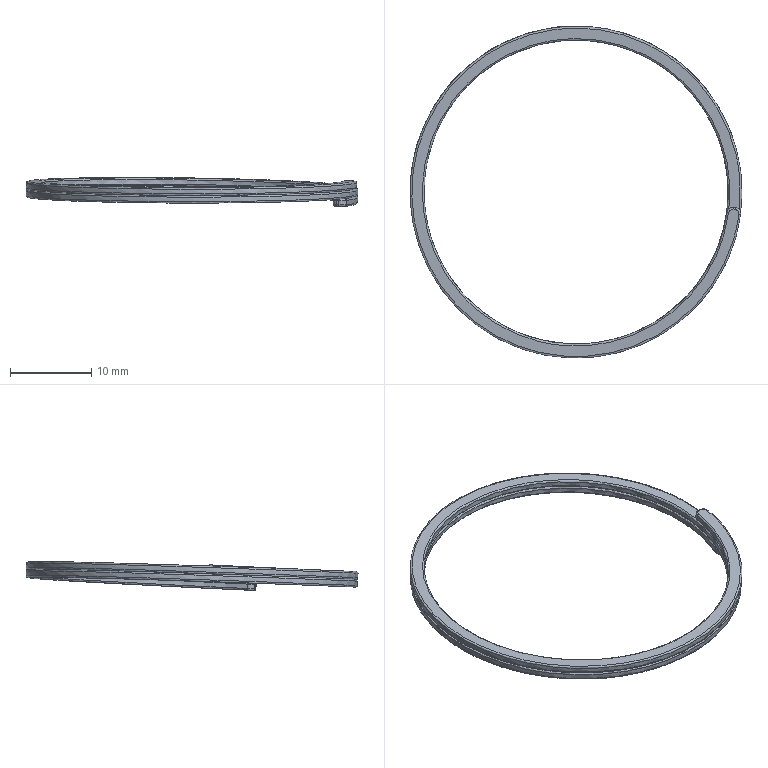Part | SolidWorks | features BaseBody 1 | 1 solid | 26 faces | box 40.908 x 40.949 x 3.578 mm | volume 397.302 mm3 | spline 24 | plane 2